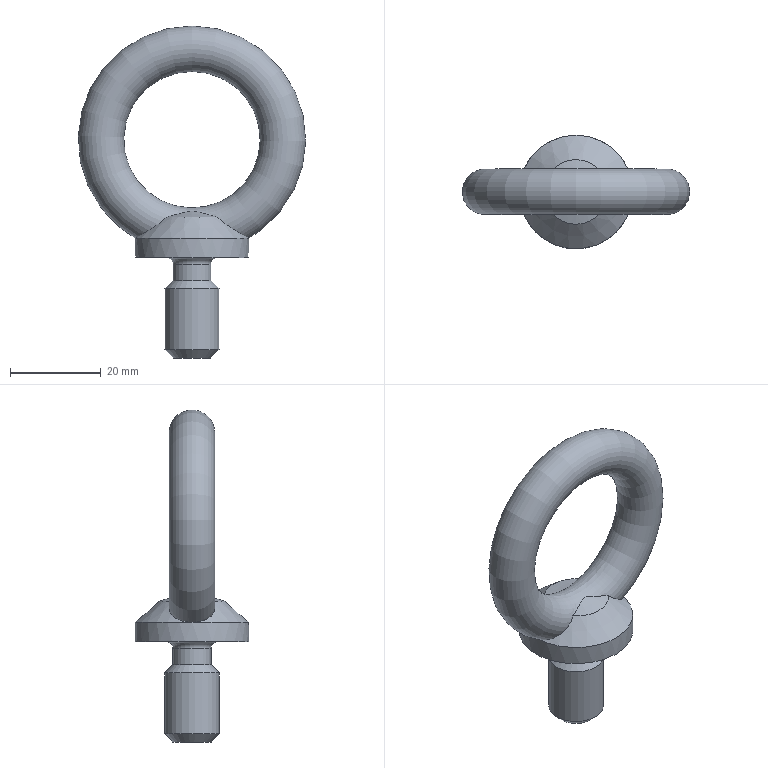Part | NX | features MAIN_BODY 2 | 1 solid | 13 faces | box 50 x 25 x 73 mm | volume 14391 mm3 | cone 6 | cylinder 3 | torus 2 | plane 2 | commonest cylinder face diameters 8.36 x1 12 x1 25 x1
STEP:
#1=CARTESIAN_POINT('',(-1280.,-175.,82.));
#2=VERTEX_POINT('',#1);
#3=VERTEX_LOOP('',#2);
#4=FACE_BOUND('',#3,.T.);
#5=CARTESIAN_POINT('',(-1274.524,-170.481,80.));
#6=VERTEX_POINT('',#5);
#7=CARTESIAN_POINT('',(-1285.476,-170.481,80.));
#8=VERTEX_POINT('',#7);
#9=CARTESIAN_POINT('',(-1274.524,-170.481,80.));
#10=CARTESIAN_POINT('',(-1275.46,-170.729,80.248));
#11=CARTESIAN_POINT('',(-1276.831,-171.224,80.621));
#12=CARTESIAN_POINT('',(-1278.576,-172.017,81.082));
#13=CARTESIAN_POINT('',(-1280.022,-172.58,81.358));
#14=CARTESIAN_POINT('',(-1281.448,-172.002,81.074));
#15=CARTESIAN_POINT('',(-1283.184,-171.22,80.618));
#16=CARTESIAN_POINT('',(-1284.545,-170.727,80.247));
#17=CARTESIAN_POINT('',(-1285.476,-170.481,80.));
#18=B_SPLINE_CURVE_WITH_KNOTS('',3,(#9,#10,#11,#12,#13,#14,#15,#16,#17),.UNSPECIFIED.,.F.,.F.,(4,1,1,1,1,1,4),(0.000000804,0.002989,0.004484,0.005978,0.007472,0.008967,0.01196),.UNSPECIFIED.);
#19=EDGE_CURVE('',#6,#8,#18,.T.);
#20=ORIENTED_EDGE('',*,*,#19,.T.);
#21=CARTESIAN_POINT('',(-1292.5,-175.,75.349));
#22=VERTEX_POINT('',#21);
#23=CARTESIAN_POINT('',(-1285.476,-170.481,80.));
#24=CARTESIAN_POINT('',(-1286.094,-170.116,79.389));
#25=CARTESIAN_POINT('',(-1287.579,-169.827,78.242));
#26=CARTESIAN_POINT('',(-1289.925,-170.455,76.766));
#27=CARTESIAN_POINT('',(-1291.927,-172.229,75.649));
#28=CARTESIAN_POINT('',(-1292.5,-174.067,75.349));
#29=CARTESIAN_POINT('',(-1292.5,-175.,75.349));
#30=B_SPLINE_CURVE_WITH_KNOTS('',3,(#23,#24,#25,#26,#27,#28,#29),.UNSPECIFIED.,.F.,.F.,(4,1,1,1,4),(0.000000303,0.00278,0.005559,0.008338,0.01112),.UNSPECIFIED.);
#31=EDGE_CURVE('',#8,#22,#30,.T.);
#32=ORIENTED_EDGE('',*,*,#31,.T.);
#33=CARTESIAN_POINT('',(-1285.476,-179.519,80.));
#34=VERTEX_POINT('',#33);
#35=CARTESIAN_POINT('',(-1292.5,-175.,75.349));
#36=CARTESIAN_POINT('',(-1292.5,-175.931,75.349));
#37=CARTESIAN_POINT('',(-1291.922,-177.78,75.652));
#38=CARTESIAN_POINT('',(-1289.92,-179.547,76.768));
#39=CARTESIAN_POINT('',(-1287.569,-180.173,78.249));
#40=CARTESIAN_POINT('',(-1286.094,-179.884,79.389));
#41=CARTESIAN_POINT('',(-1285.476,-179.519,80.));
#42=B_SPLINE_CURVE_WITH_KNOTS('',3,(#35,#36,#37,#38,#39,#40,#41),.UNSPECIFIED.,.F.,.F.,(4,1,1,1,4),(0.01112,0.01389,0.01666,0.01943,0.02221),.UNSPECIFIED.);
#43=EDGE_CURVE('',#22,#34,#42,.T.);
#44=ORIENTED_EDGE('',*,*,#43,.T.);
#45=CARTESIAN_POINT('',(-1274.524,-179.519,80.));
#46=VERTEX_POINT('',#45);
#47=CARTESIAN_POINT('',(-1285.476,-179.519,80.));
#48=CARTESIAN_POINT('',(-1284.54,-179.271,80.248));
#49=CARTESIAN_POINT('',(-1283.169,-178.776,80.621));
#50=CARTESIAN_POINT('',(-1281.424,-177.983,81.082));
#51=CARTESIAN_POINT('',(-1279.978,-177.42,81.358));
#52=CARTESIAN_POINT('',(-1278.552,-177.998,81.074));
#53=CARTESIAN_POINT('',(-1276.816,-178.78,80.618));
#54=CARTESIAN_POINT('',(-1275.455,-179.273,80.247));
#55=CARTESIAN_POINT('',(-1274.524,-179.519,80.));
#56=B_SPLINE_CURVE_WITH_KNOTS('',3,(#47,#48,#49,#50,#51,#52,#53,#54,#55),.UNSPECIFIED.,.F.,.F.,(4,1,1,1,1,1,4),(0.000000804,0.002989,0.004484,0.005978,0.007472,0.008967,0.01196),.UNSPECIFIED.);
#57=EDGE_CURVE('',#34,#46,#56,.T.);
#58=ORIENTED_EDGE('',*,*,#57,.T.);
#59=CARTESIAN_POINT('',(-1267.5,-175.,75.349));
#60=VERTEX_POINT('',#59);
#61=CARTESIAN_POINT('',(-1274.524,-179.519,80.));
#62=CARTESIAN_POINT('',(-1273.906,-179.884,79.389));
#63=CARTESIAN_POINT('',(-1272.421,-180.173,78.242));
#64=CARTESIAN_POINT('',(-1270.075,-179.545,76.766));
#65=CARTESIAN_POINT('',(-1268.073,-177.771,75.649));
#66=CARTESIAN_POINT('',(-1267.5,-175.933,75.349));
#67=CARTESIAN_POINT('',(-1267.5,-175.,75.349));
#68=B_SPLINE_CURVE_WITH_KNOTS('',3,(#61,#62,#63,#64,#65,#66,#67),.UNSPECIFIED.,.F.,.F.,(4,1,1,1,4),(0.000000303,0.00278,0.005559,0.008338,0.01112),.UNSPECIFIED.);
#69=EDGE_CURVE('',#46,#60,#68,.T.);
#70=ORIENTED_EDGE('',*,*,#69,.T.);
#71=CARTESIAN_POINT('',(-1267.5,-175.,75.349));
#72=CARTESIAN_POINT('',(-1267.5,-174.069,75.349));
#73=CARTESIAN_POINT('',(-1268.078,-172.22,75.652));
#74=CARTESIAN_POINT('',(-1270.08,-170.453,76.768));
#75=CARTESIAN_POINT('',(-1272.431,-169.827,78.249));
#76=CARTESIAN_POINT('',(-1273.906,-170.116,79.389));
#77=CARTESIAN_POINT('',(-1274.524,-170.481,80.));
#78=B_SPLINE_CURVE_WITH_KNOTS('',3,(#71,#72,#73,#74,#75,#76,#77),.UNSPECIFIED.,.F.,.F.,(4,1,1,1,4),(0.01112,0.01389,0.01666,0.01943,0.02221),.UNSPECIFIED.);
#79=EDGE_CURVE('',#60,#6,#78,.T.);
#80=ORIENTED_EDGE('',*,*,#79,.T.);
#81=EDGE_LOOP('',(#20,#32,#44,#58,#70,#80));
#82=FACE_BOUND('',#81,.T.);
#83=CARTESIAN_POINT('',(-1280.,-175.,97.));
#84=DIRECTION('',(0.,-1.,0.));
#85=DIRECTION('',(0.,0.,1.));
#86=AXIS2_PLACEMENT_3D('',#83,#84,#85);
#87=TOROIDAL_SURFACE('',#86,20.,5.);
#88=ADVANCED_FACE('',(#4,#82),#87,.T.);
#89=CARTESIAN_POINT('',(-1280.,-169.42,71.));
#90=VERTEX_POINT('',#89);
#91=CARTESIAN_POINT('',(-1280.,-175.,71.));
#92=DIRECTION('',(0.,0.,-1.));
#93=DIRECTION('',(0.,1.,0.));
#94=AXIS2_PLACEMENT_3D('',#91,#92,#93);
#95=CIRCLE('',#94,5.58);
#96=EDGE_CURVE('',#90,#90,#95,.T.);
#97=ORIENTED_EDGE('',*,*,#96,.F.);
#98=EDGE_LOOP('',(#97));
#99=FACE_BOUND('',#98,.T.);
#100=CARTESIAN_POINT('',(-1280.,-162.5,71.));
#101=VERTEX_POINT('',#100);
#102=CARTESIAN_POINT('',(-1280.,-175.,71.));
#103=DIRECTION('',(0.,0.,-1.));
#104=DIRECTION('',(0.,1.,0.));
#105=AXIS2_PLACEMENT_3D('',#102,#103,#104);
#106=CIRCLE('',#105,12.5);
#107=EDGE_CURVE('',#101,#101,#106,.T.);
#108=ORIENTED_EDGE('',*,*,#107,.T.);
#109=EDGE_LOOP('',(#108));
#110=FACE_BOUND('',#109,.T.);
#111=CARTESIAN_POINT('',(-1280.,-175.,71.));
#112=DIRECTION('',(0.,0.,1.));
#113=DIRECTION('',(0.,1.,0.));
#114=AXIS2_PLACEMENT_3D('',#111,#112,#113);
#115=PLANE('',#114);
#116=ADVANCED_FACE('',(#99,#110),#115,.F.);
#117=CARTESIAN_POINT('',(-1280.,-175.,80.));
#118=DIRECTION('',(0.,0.,-1.));
#119=DIRECTION('',(0.,1.,0.));
#120=AXIS2_PLACEMENT_3D('',#117,#118,#119);
#121=CIRCLE('',#120,7.1);
#122=EDGE_CURVE('',#46,#34,#121,.T.);
#123=ORIENTED_EDGE('',*,*,#122,.T.);
#124=ORIENTED_EDGE('',*,*,#43,.F.);
#125=CARTESIAN_POINT('',(-1280.,-175.,75.349));
#126=DIRECTION('',(0.,0.,-1.));
#127=DIRECTION('',(0.,1.,0.));
#128=AXIS2_PLACEMENT_3D('',#125,#126,#127);
#129=CIRCLE('',#128,12.5);
#130=EDGE_CURVE('',#60,#22,#129,.T.);
#131=ORIENTED_EDGE('',*,*,#130,.F.);
#132=ORIENTED_EDGE('',*,*,#69,.F.);
#133=EDGE_LOOP('',(#123,#124,#131,#132));
#134=FACE_BOUND('',#133,.T.);
#135=CARTESIAN_POINT('',(-1280.,-175.,75.349));
#136=DIRECTION('',(0.,0.,-1.));
#137=DIRECTION('',(0.,-1.,0.));
#138=AXIS2_PLACEMENT_3D('',#135,#136,#137);
#139=CONICAL_SURFACE('',#138,12.5,0.8598);
#140=ADVANCED_FACE('',(#134),#139,.T.);
#141=CARTESIAN_POINT('',(-1280.,-175.,75.349));
#142=DIRECTION('',(0.,0.,-1.));
#143=DIRECTION('',(0.,1.,0.));
#144=AXIS2_PLACEMENT_3D('',#141,#142,#143);
#145=CIRCLE('',#144,12.5);
#146=EDGE_CURVE('',#22,#60,#145,.T.);
#147=ORIENTED_EDGE('',*,*,#146,.F.);
#148=ORIENTED_EDGE('',*,*,#31,.F.);
#149=CARTESIAN_POINT('',(-1280.,-175.,80.));
#150=DIRECTION('',(0.,0.,-1.));
#151=DIRECTION('',(0.,1.,0.));
#152=AXIS2_PLACEMENT_3D('',#149,#150,#151);
#153=CIRCLE('',#152,7.1);
#154=EDGE_CURVE('',#8,#6,#153,.T.);
#155=ORIENTED_EDGE('',*,*,#154,.T.);
#156=ORIENTED_EDGE('',*,*,#79,.F.);
#157=EDGE_LOOP('',(#147,#148,#155,#156));
#158=FACE_BOUND('',#157,.T.);
#159=CARTESIAN_POINT('',(-1280.,-175.,75.349));
#160=DIRECTION('',(0.,0.,-1.));
#161=DIRECTION('',(0.,-1.,0.));
#162=AXIS2_PLACEMENT_3D('',#159,#160,#161);
#163=CONICAL_SURFACE('',#162,12.5,0.8598);
#164=ADVANCED_FACE('',(#158),#163,.T.);
#165=ORIENTED_EDGE('',*,*,#130,.T.);
#166=ORIENTED_EDGE('',*,*,#146,.T.);
#167=EDGE_LOOP('',(#165,#166));
#168=FACE_BOUND('',#167,.T.);
#169=ORIENTED_EDGE('',*,*,#107,.F.);
#170=EDGE_LOOP('',(#169));
#171=FACE_BOUND('',#170,.T.);
#172=CARTESIAN_POINT('',(-1280.,-175.,62.));
#173=DIRECTION('',(0.,0.,1.));
#174=DIRECTION('',(0.,1.,0.));
#175=AXIS2_PLACEMENT_3D('',#172,#173,#174);
#176=CYLINDRICAL_SURFACE('',#175,12.5);
#177=ADVANCED_FACE('',(#168,#171),#176,.T.);
#178=CARTESIAN_POINT('',(-1280.,-170.82,69.6));
#179=VERTEX_POINT('',#178);
#180=CARTESIAN_POINT('',(-1280.,-175.,69.6));
#181=DIRECTION('',(0.,0.,-1.));
#182=DIRECTION('',(0.,1.,0.));
#183=AXIS2_PLACEMENT_3D('',#180,#181,#182);
#184=CIRCLE('',#183,4.18);
#185=EDGE_CURVE('',#179,#179,#184,.F.);
#186=ORIENTED_EDGE('',*,*,#185,.F.);
#187=EDGE_LOOP('',(#186));
#188=FACE_BOUND('',#187,.T.);
#189=CARTESIAN_POINT('',(-1280.,-179.18,66.));
#190=VERTEX_POINT('',#189);
#191=CARTESIAN_POINT('',(-1280.,-175.,66.));
#192=DIRECTION('',(0.,0.,1.));
#193=DIRECTION('',(0.,-1.,0.));
#194=AXIS2_PLACEMENT_3D('',#191,#192,#193);
#195=CIRCLE('',#194,4.18);
#196=EDGE_CURVE('',#190,#190,#195,.F.);
#197=ORIENTED_EDGE('',*,*,#196,.F.);
#198=EDGE_LOOP('',(#197));
#199=FACE_BOUND('',#198,.T.);
#200=CARTESIAN_POINT('',(-1280.,-175.,71.));
#201=DIRECTION('',(0.,0.,-1.));
#202=DIRECTION('',(0.,-1.,0.));
#203=AXIS2_PLACEMENT_3D('',#200,#201,#202);
#204=CYLINDRICAL_SURFACE('',#203,4.18);
#205=ADVANCED_FACE('',(#188,#199),#204,.T.);
#206=CARTESIAN_POINT('',(-1280.,-181.,64.18));
#207=VERTEX_POINT('',#206);
#208=CARTESIAN_POINT('',(-1280.,-175.,64.18));
#209=DIRECTION('',(0.,0.,1.));
#210=DIRECTION('',(0.,-1.,0.));
#211=AXIS2_PLACEMENT_3D('',#208,#209,#210);
#212=CIRCLE('',#211,6.);
#213=EDGE_CURVE('',#207,#207,#212,.T.);
#214=ORIENTED_EDGE('',*,*,#213,.F.);
#215=EDGE_LOOP('',(#214));
#216=FACE_BOUND('',#215,.T.);
#217=CARTESIAN_POINT('',(-1280.,-181.,50.82));
#218=VERTEX_POINT('',#217);
#219=CARTESIAN_POINT('',(-1280.,-175.,50.82));
#220=DIRECTION('',(0.,0.,1.));
#221=DIRECTION('',(0.,-1.,0.));
#222=AXIS2_PLACEMENT_3D('',#219,#220,#221);
#223=CIRCLE('',#222,6.);
#224=EDGE_CURVE('',#218,#218,#223,.F.);
#225=ORIENTED_EDGE('',*,*,#224,.F.);
#226=EDGE_LOOP('',(#225));
#227=FACE_BOUND('',#226,.T.);
#228=CARTESIAN_POINT('',(-1280.,-175.,49.));
#229=DIRECTION('',(0.,0.,1.));
#230=DIRECTION('',(0.,1.,0.));
#231=AXIS2_PLACEMENT_3D('',#228,#229,#230);
#232=CYLINDRICAL_SURFACE('',#231,6.);
#233=ADVANCED_FACE('',(#216,#227),#232,.T.);
#234=CARTESIAN_POINT('',(-1280.,-179.18,49.));
#235=VERTEX_POINT('',#234);
#236=CARTESIAN_POINT('',(-1280.,-175.,49.));
#237=DIRECTION('',(0.,0.,1.));
#238=DIRECTION('',(0.,-1.,0.));
#239=AXIS2_PLACEMENT_3D('',#236,#237,#238);
#240=CIRCLE('',#239,4.18);
#241=EDGE_CURVE('',#235,#235,#240,.T.);
#242=ORIENTED_EDGE('',*,*,#241,.F.);
#243=EDGE_LOOP('',(#242));
#244=FACE_BOUND('',#243,.T.);
#245=CARTESIAN_POINT('',(-1280.,-175.,49.));
#246=DIRECTION('',(0.,0.,-1.));
#247=DIRECTION('',(0.,-1.,0.));
#248=AXIS2_PLACEMENT_3D('',#245,#246,#247);
#249=PLANE('',#248);
#250=ADVANCED_FACE('',(#244),#249,.T.);
#251=ORIENTED_EDGE('',*,*,#224,.T.);
#252=EDGE_LOOP('',(#251));
#253=FACE_BOUND('',#252,.T.);
#254=ORIENTED_EDGE('',*,*,#241,.T.);
#255=EDGE_LOOP('',(#254));
#256=FACE_BOUND('',#255,.T.);
#257=CARTESIAN_POINT('',(-1280.,-175.,49.));
#258=DIRECTION('',(0.,0.,1.));
#259=DIRECTION('',(0.,1.,0.));
#260=AXIS2_PLACEMENT_3D('',#257,#258,#259);
#261=CONICAL_SURFACE('',#260,4.18,0.7854);
#262=ADVANCED_FACE('',(#253,#256),#261,.T.);
#263=ORIENTED_EDGE('',*,*,#196,.T.);
#264=EDGE_LOOP('',(#263));
#265=FACE_BOUND('',#264,.T.);
#266=ORIENTED_EDGE('',*,*,#213,.T.);
#267=EDGE_LOOP('',(#266));
#268=FACE_BOUND('',#267,.T.);
#269=CARTESIAN_POINT('',(-1280.,-175.,64.18));
#270=DIRECTION('',(0.,0.,-1.));
#271=DIRECTION('',(0.,-1.,0.));
#272=AXIS2_PLACEMENT_3D('',#269,#270,#271);
#273=CONICAL_SURFACE('',#272,6.,0.7854);
#274=ADVANCED_FACE('',(#265,#268),#273,.T.);
#275=ORIENTED_EDGE('',*,*,#96,.T.);
#276=EDGE_LOOP('',(#275));
#277=FACE_BOUND('',#276,.T.);
#278=ORIENTED_EDGE('',*,*,#185,.T.);
#279=EDGE_LOOP('',(#278));
#280=FACE_BOUND('',#279,.T.);
#281=CARTESIAN_POINT('',(-1280.,-175.,69.6));
#282=DIRECTION('',(0.,0.,1.));
#283=DIRECTION('',(0.,1.,0.));
#284=AXIS2_PLACEMENT_3D('',#281,#282,#283);
#285=TOROIDAL_SURFACE('',#284,5.58,1.4);
#286=ADVANCED_FACE('',(#277,#280),#285,.F.);
#287=ORIENTED_EDGE('',*,*,#154,.F.);
#288=ORIENTED_EDGE('',*,*,#19,.F.);
#289=EDGE_LOOP('',(#287,#288));
#290=FACE_BOUND('',#289,.T.);
#291=CARTESIAN_POINT('',(-1280.,-175.,80.));
#292=DIRECTION('',(0.,0.,-1.));
#293=DIRECTION('',(0.,-1.,0.));
#294=AXIS2_PLACEMENT_3D('',#291,#292,#293);
#295=CONICAL_SURFACE('',#294,7.1,1.296);
#296=ADVANCED_FACE('',(#290),#295,.T.);
#297=ORIENTED_EDGE('',*,*,#122,.F.);
#298=ORIENTED_EDGE('',*,*,#57,.F.);
#299=EDGE_LOOP('',(#297,#298));
#300=FACE_BOUND('',#299,.T.);
#301=CARTESIAN_POINT('',(-1280.,-175.,80.));
#302=DIRECTION('',(0.,0.,-1.));
#303=DIRECTION('',(0.,-1.,0.));
#304=AXIS2_PLACEMENT_3D('',#301,#302,#303);
#305=CONICAL_SURFACE('',#304,7.1,1.296);
#306=ADVANCED_FACE('',(#300),#305,.T.);
#307=CLOSED_SHELL('',(#88,#116,#140,#164,#177,#205,#233,#250,#262,#274,#286,#296,#306));
#308=MANIFOLD_SOLID_BREP('',#307);
#309=(LENGTH_UNIT()NAMED_UNIT(*)SI_UNIT(.MILLI.,.METRE.));
#310=UNCERTAINTY_MEASURE_WITH_UNIT(LENGTH_MEASURE(0.0508),#309,'','');
#311=(NAMED_UNIT(*)PLANE_ANGLE_UNIT()SI_UNIT($,.RADIAN.));
#312=(NAMED_UNIT(*)SI_UNIT($,.STERADIAN.)SOLID_ANGLE_UNIT());
#313=(GEOMETRIC_REPRESENTATION_CONTEXT(3)GLOBAL_UNCERTAINTY_ASSIGNED_CONTEXT((#310))GLOBAL_UNIT_ASSIGNED_CONTEXT((#309,#311,#312))REPRESENTATION_CONTEXT('',''));
#314=ADVANCED_BREP_SHAPE_REPRESENTATION('',(#308),#313);